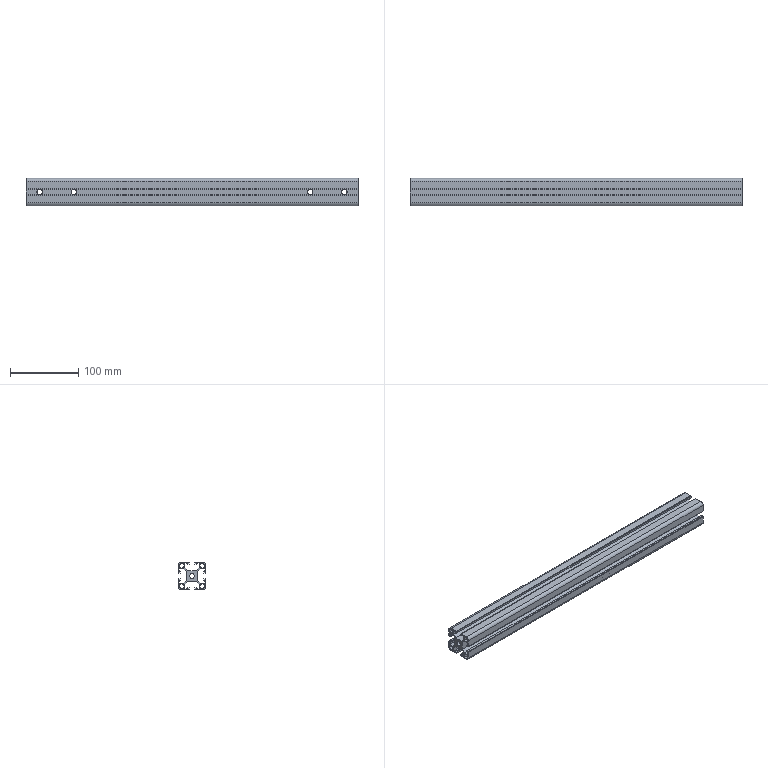Part | 1 solid | 120 faces | box 485 x 40 x 40 mm | volume 277449 mm3 | plane 94 | cylinder 26 | commonest cylinder face diameters 6.8 x10 8.2 x8 5 x4 9 x4